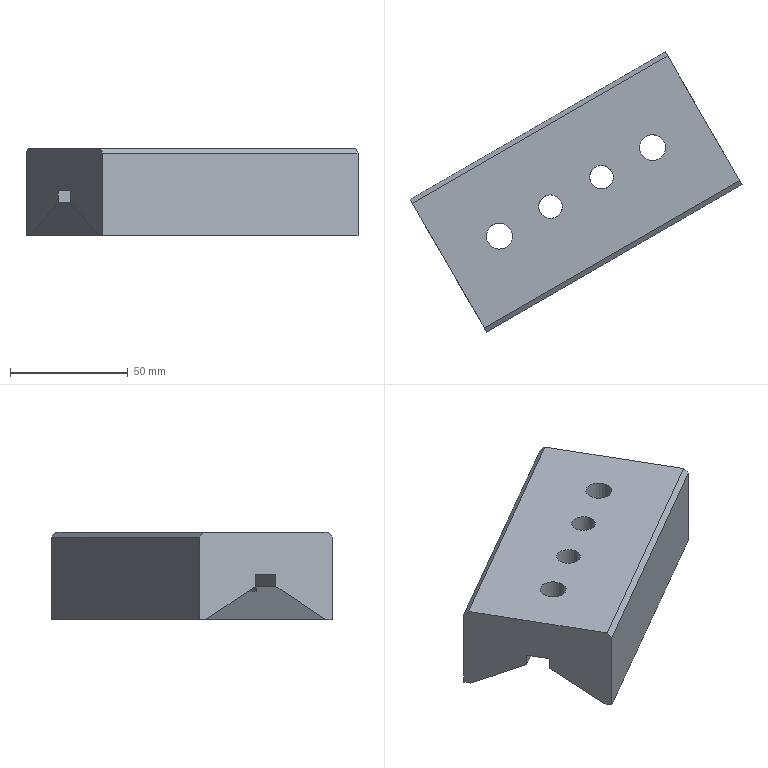Part | NX | features solid 2 | 1 solid | 30 faces | box 140.753 x 118.792 x 37 mm | volume 223802 mm3 | plane 24 | cylinder 6 | commonest cylinder face diameters 10 x2 11 x2 17.5 x2
STEP:
#1=CARTESIAN_POINT('',(-902.48,110.974,-228.));
#2=VERTEX_POINT('',#1);
#3=CARTESIAN_POINT('',(-917.912,102.065,-228.));
#4=VERTEX_POINT('',#3);
#5=CARTESIAN_POINT('',(-902.48,110.974,-228.));
#6=DIRECTION('',(-0.866,-0.5,0.));
#7=VECTOR('',#6,1000.);
#8=LINE('',#5,#7);
#9=EDGE_CURVE('',#2,#4,#8,.T.);
#10=ORIENTED_EDGE('',*,*,#9,.F.);
#11=CARTESIAN_POINT('',(-902.48,110.974,-232.887));
#12=VERTEX_POINT('',#11);
#13=CARTESIAN_POINT('',(-902.48,110.974,-228.));
#14=DIRECTION('',(0.,0.,-1.));
#15=VECTOR('',#14,1000.);
#16=LINE('',#13,#15);
#17=EDGE_CURVE('',#2,#12,#16,.T.);
#18=ORIENTED_EDGE('',*,*,#17,.T.);
#19=CARTESIAN_POINT('',(-917.912,102.065,-232.887));
#20=VERTEX_POINT('',#19);
#21=CARTESIAN_POINT('',(-902.48,110.974,-232.887));
#22=DIRECTION('',(-0.866,-0.5,0.));
#23=VECTOR('',#22,1000.);
#24=LINE('',#21,#23);
#25=EDGE_CURVE('',#12,#20,#24,.T.);
#26=ORIENTED_EDGE('',*,*,#25,.T.);
#27=CARTESIAN_POINT('',(-917.912,102.065,-220.));
#28=DIRECTION('',(0.,0.,-1.));
#29=VECTOR('',#28,1000.);
#30=LINE('',#27,#29);
#31=EDGE_CURVE('',#4,#20,#30,.T.);
#32=ORIENTED_EDGE('',*,*,#31,.F.);
#33=EDGE_LOOP('',(#10,#18,#26,#32));
#34=FACE_BOUND('',#33,.T.);
#35=CARTESIAN_POINT('',(-902.48,110.974,-228.));
#36=DIRECTION('',(0.5,-0.866,0.));
#37=DIRECTION('',(0.,0.,1.));
#38=AXIS2_PLACEMENT_3D('',#35,#36,#37);
#39=PLANE('',#38);
#40=ADVANCED_FACE('',(#34),#39,.F.);
#41=CARTESIAN_POINT('',(-930.349,94.884,-228.));
#42=VERTEX_POINT('',#41);
#43=CARTESIAN_POINT('',(-945.781,85.974,-228.));
#44=VERTEX_POINT('',#43);
#45=CARTESIAN_POINT('',(-902.48,110.974,-228.));
#46=DIRECTION('',(-0.866,-0.5,0.));
#47=VECTOR('',#46,1000.);
#48=LINE('',#45,#47);
#49=EDGE_CURVE('',#42,#44,#48,.T.);
#50=ORIENTED_EDGE('',*,*,#49,.T.);
#51=CARTESIAN_POINT('',(-950.781,94.634,-228.));
#52=VERTEX_POINT('',#51);
#53=CARTESIAN_POINT('',(-948.281,90.304,-228.));
#54=DIRECTION('',(0.,0.,-1.));
#55=DIRECTION('',(0.866,0.5,0.));
#56=AXIS2_PLACEMENT_3D('',#53,#54,#55);
#57=CIRCLE('',#56,5.);
#58=EDGE_CURVE('',#52,#44,#57,.T.);
#59=ORIENTED_EDGE('',*,*,#58,.F.);
#60=CARTESIAN_POINT('',(-935.349,103.544,-228.));
#61=VERTEX_POINT('',#60);
#62=CARTESIAN_POINT('',(-907.48,119.634,-228.));
#63=DIRECTION('',(-0.866,-0.5,0.));
#64=VECTOR('',#63,1000.);
#65=LINE('',#62,#64);
#66=EDGE_CURVE('',#61,#52,#65,.T.);
#67=ORIENTED_EDGE('',*,*,#66,.F.);
#68=CARTESIAN_POINT('',(-926.631,102.804,-228.));
#69=DIRECTION('',(0.,0.,-1.));
#70=DIRECTION('',(0.866,0.5,0.));
#71=AXIS2_PLACEMENT_3D('',#68,#69,#70);
#72=CIRCLE('',#71,8.75);
#73=EDGE_CURVE('',#42,#61,#72,.T.);
#74=ORIENTED_EDGE('',*,*,#73,.F.);
#75=EDGE_LOOP('',(#50,#59,#67,#74));
#76=FACE_BOUND('',#75,.T.);
#77=CARTESIAN_POINT('',(-907.48,119.634,-228.));
#78=DIRECTION('',(0.,0.,1.));
#79=DIRECTION('',(0.866,0.5,0.));
#80=AXIS2_PLACEMENT_3D('',#77,#78,#79);
#81=PLANE('',#80);
#82=ADVANCED_FACE('',(#76),#81,.F.);
#83=ORIENTED_EDGE('',*,*,#66,.T.);
#84=CARTESIAN_POINT('',(-972.432,82.134,-228.));
#85=VERTEX_POINT('',#84);
#86=CARTESIAN_POINT('',(-907.48,119.634,-228.));
#87=DIRECTION('',(-0.866,-0.5,0.));
#88=VECTOR('',#87,1000.);
#89=LINE('',#86,#88);
#90=EDGE_CURVE('',#52,#85,#89,.T.);
#91=ORIENTED_EDGE('',*,*,#90,.T.);
#92=CARTESIAN_POINT('',(-987.864,73.225,-228.));
#93=VERTEX_POINT('',#92);
#94=CARTESIAN_POINT('',(-907.48,119.634,-228.));
#95=DIRECTION('',(-0.866,-0.5,0.));
#96=VECTOR('',#95,1000.);
#97=LINE('',#94,#96);
#98=EDGE_CURVE('',#85,#93,#97,.T.);
#99=ORIENTED_EDGE('',*,*,#98,.T.);
#100=CARTESIAN_POINT('',(-987.864,73.225,-232.887));
#101=VERTEX_POINT('',#100);
#102=CARTESIAN_POINT('',(-987.864,73.225,-220.));
#103=DIRECTION('',(0.,0.,-1.));
#104=VECTOR('',#103,1000.);
#105=LINE('',#102,#104);
#106=EDGE_CURVE('',#101,#93,#105,.F.);
#107=ORIENTED_EDGE('',*,*,#106,.F.);
#108=CARTESIAN_POINT('',(-935.349,103.544,-232.887));
#109=VERTEX_POINT('',#108);
#110=CARTESIAN_POINT('',(-907.48,119.634,-232.887));
#111=DIRECTION('',(-0.866,-0.5,0.));
#112=VECTOR('',#111,1000.);
#113=LINE('',#110,#112);
#114=EDGE_CURVE('',#109,#101,#113,.T.);
#115=ORIENTED_EDGE('',*,*,#114,.F.);
#116=CARTESIAN_POINT('',(-935.349,103.544,-220.));
#117=DIRECTION('',(0.,0.,-1.));
#118=VECTOR('',#117,1000.);
#119=LINE('',#116,#118);
#120=EDGE_CURVE('',#61,#109,#119,.T.);
#121=ORIENTED_EDGE('',*,*,#120,.F.);
#122=EDGE_LOOP('',(#83,#91,#99,#107,#115,#121));
#123=FACE_BOUND('',#122,.T.);
#124=CARTESIAN_POINT('',(-907.48,119.634,-232.887));
#125=DIRECTION('',(-0.5,0.866,0.));
#126=DIRECTION('',(0.,0.,-1.));
#127=AXIS2_PLACEMENT_3D('',#124,#125,#126);
#128=PLANE('',#127);
#129=ADVANCED_FACE('',(#123),#128,.F.);
#130=CARTESIAN_POINT('',(-967.432,73.474,-228.));
#131=VERTEX_POINT('',#130);
#132=CARTESIAN_POINT('',(-902.48,110.974,-228.));
#133=DIRECTION('',(-0.866,-0.5,0.));
#134=VECTOR('',#133,1000.);
#135=LINE('',#132,#134);
#136=EDGE_CURVE('',#44,#131,#135,.T.);
#137=ORIENTED_EDGE('',*,*,#136,.T.);
#138=CARTESIAN_POINT('',(-969.932,77.804,-228.));
#139=DIRECTION('',(0.,0.,-1.));
#140=DIRECTION('',(0.866,0.5,0.));
#141=AXIS2_PLACEMENT_3D('',#138,#139,#140);
#142=CIRCLE('',#141,5.);
#143=EDGE_CURVE('',#85,#131,#142,.T.);
#144=ORIENTED_EDGE('',*,*,#143,.F.);
#145=ORIENTED_EDGE('',*,*,#90,.F.);
#146=CARTESIAN_POINT('',(-948.281,90.304,-228.));
#147=DIRECTION('',(0.,0.,-1.));
#148=DIRECTION('',(0.866,0.5,0.));
#149=AXIS2_PLACEMENT_3D('',#146,#147,#148);
#150=CIRCLE('',#149,5.);
#151=EDGE_CURVE('',#44,#52,#150,.T.);
#152=ORIENTED_EDGE('',*,*,#151,.F.);
#153=EDGE_LOOP('',(#137,#144,#145,#152));
#154=FACE_BOUND('',#153,.T.);
#155=CARTESIAN_POINT('',(-907.48,119.634,-228.));
#156=DIRECTION('',(0.,0.,1.));
#157=DIRECTION('',(0.866,0.5,0.));
#158=AXIS2_PLACEMENT_3D('',#155,#156,#157);
#159=PLANE('',#158);
#160=ADVANCED_FACE('',(#154),#159,.F.);
#161=CARTESIAN_POINT('',(-982.864,64.565,-228.));
#162=VERTEX_POINT('',#161);
#163=CARTESIAN_POINT('',(-902.48,110.974,-228.));
#164=DIRECTION('',(-0.866,-0.5,0.));
#165=VECTOR('',#164,1000.);
#166=LINE('',#163,#165);
#167=EDGE_CURVE('',#131,#162,#166,.T.);
#168=ORIENTED_EDGE('',*,*,#167,.T.);
#169=CARTESIAN_POINT('',(-991.583,65.304,-228.));
#170=DIRECTION('',(0.,0.,-1.));
#171=DIRECTION('',(0.866,0.5,0.));
#172=AXIS2_PLACEMENT_3D('',#169,#170,#171);
#173=CIRCLE('',#172,8.75);
#174=EDGE_CURVE('',#93,#162,#173,.T.);
#175=ORIENTED_EDGE('',*,*,#174,.F.);
#176=ORIENTED_EDGE('',*,*,#98,.F.);
#177=CARTESIAN_POINT('',(-969.932,77.804,-228.));
#178=DIRECTION('',(0.,0.,-1.));
#179=DIRECTION('',(0.866,0.5,0.));
#180=AXIS2_PLACEMENT_3D('',#177,#178,#179);
#181=CIRCLE('',#180,5.);
#182=EDGE_CURVE('',#131,#85,#181,.T.);
#183=ORIENTED_EDGE('',*,*,#182,.F.);
#184=EDGE_LOOP('',(#168,#175,#176,#183));
#185=FACE_BOUND('',#184,.T.);
#186=CARTESIAN_POINT('',(-907.48,119.634,-228.));
#187=DIRECTION('',(0.,0.,1.));
#188=DIRECTION('',(0.866,0.5,0.));
#189=AXIS2_PLACEMENT_3D('',#186,#187,#188);
#190=PLANE('',#189);
#191=ADVANCED_FACE('',(#185),#190,.F.);
#192=CARTESIAN_POINT('',(-930.349,94.884,-232.887));
#193=VERTEX_POINT('',#192);
#194=CARTESIAN_POINT('',(-982.864,64.565,-232.887));
#195=VERTEX_POINT('',#194);
#196=CARTESIAN_POINT('',(-902.48,110.974,-232.887));
#197=DIRECTION('',(-0.866,-0.5,0.));
#198=VECTOR('',#197,1000.);
#199=LINE('',#196,#198);
#200=EDGE_CURVE('',#193,#195,#199,.T.);
#201=ORIENTED_EDGE('',*,*,#200,.T.);
#202=CARTESIAN_POINT('',(-982.864,64.565,-220.));
#203=DIRECTION('',(0.,0.,-1.));
#204=VECTOR('',#203,1000.);
#205=LINE('',#202,#204);
#206=EDGE_CURVE('',#162,#195,#205,.T.);
#207=ORIENTED_EDGE('',*,*,#206,.F.);
#208=ORIENTED_EDGE('',*,*,#167,.F.);
#209=ORIENTED_EDGE('',*,*,#136,.F.);
#210=ORIENTED_EDGE('',*,*,#49,.F.);
#211=CARTESIAN_POINT('',(-930.349,94.884,-220.));
#212=DIRECTION('',(0.,0.,-1.));
#213=VECTOR('',#212,1000.);
#214=LINE('',#211,#213);
#215=EDGE_CURVE('',#193,#42,#214,.F.);
#216=ORIENTED_EDGE('',*,*,#215,.F.);
#217=EDGE_LOOP('',(#201,#207,#208,#209,#210,#216));
#218=FACE_BOUND('',#217,.T.);
#219=CARTESIAN_POINT('',(-902.48,110.974,-228.));
#220=DIRECTION('',(0.5,-0.866,0.));
#221=DIRECTION('',(0.,0.,1.));
#222=AXIS2_PLACEMENT_3D('',#219,#220,#221);
#223=PLANE('',#222);
#224=ADVANCED_FACE('',(#218),#223,.F.);
#225=CARTESIAN_POINT('',(-995.301,57.384,-228.));
#226=VERTEX_POINT('',#225);
#227=CARTESIAN_POINT('',(-1010.733,48.474,-228.));
#228=VERTEX_POINT('',#227);
#229=CARTESIAN_POINT('',(-902.48,110.974,-228.));
#230=DIRECTION('',(-0.866,-0.5,0.));
#231=VECTOR('',#230,1000.);
#232=LINE('',#229,#231);
#233=EDGE_CURVE('',#226,#228,#232,.T.);
#234=ORIENTED_EDGE('',*,*,#233,.T.);
#235=CARTESIAN_POINT('',(-1015.733,57.134,-228.));
#236=VERTEX_POINT('',#235);
#237=CARTESIAN_POINT('',(-1015.733,57.134,-228.));
#238=DIRECTION('',(0.5,-0.866,0.));
#239=VECTOR('',#238,1000.);
#240=LINE('',#237,#239);
#241=EDGE_CURVE('',#236,#228,#240,.T.);
#242=ORIENTED_EDGE('',*,*,#241,.F.);
#243=CARTESIAN_POINT('',(-1000.301,66.044,-228.));
#244=VERTEX_POINT('',#243);
#245=CARTESIAN_POINT('',(-907.48,119.634,-228.));
#246=DIRECTION('',(-0.866,-0.5,0.));
#247=VECTOR('',#246,1000.);
#248=LINE('',#245,#247);
#249=EDGE_CURVE('',#244,#236,#248,.T.);
#250=ORIENTED_EDGE('',*,*,#249,.F.);
#251=CARTESIAN_POINT('',(-991.583,65.304,-228.));
#252=DIRECTION('',(0.,0.,-1.));
#253=DIRECTION('',(0.866,0.5,0.));
#254=AXIS2_PLACEMENT_3D('',#251,#252,#253);
#255=CIRCLE('',#254,8.75);
#256=EDGE_CURVE('',#226,#244,#255,.T.);
#257=ORIENTED_EDGE('',*,*,#256,.F.);
#258=EDGE_LOOP('',(#234,#242,#250,#257));
#259=FACE_BOUND('',#258,.T.);
#260=CARTESIAN_POINT('',(-907.48,119.634,-228.));
#261=DIRECTION('',(0.,0.,1.));
#262=DIRECTION('',(0.866,0.5,0.));
#263=AXIS2_PLACEMENT_3D('',#260,#261,#262);
#264=PLANE('',#263);
#265=ADVANCED_FACE('',(#259),#264,.F.);
#266=ORIENTED_EDGE('',*,*,#249,.T.);
#267=CARTESIAN_POINT('',(-1015.733,57.134,-232.887));
#268=VERTEX_POINT('',#267);
#269=CARTESIAN_POINT('',(-1015.733,57.134,-232.887));
#270=DIRECTION('',(0.,0.,1.));
#271=VECTOR('',#270,1000.);
#272=LINE('',#269,#271);
#273=EDGE_CURVE('',#268,#236,#272,.T.);
#274=ORIENTED_EDGE('',*,*,#273,.F.);
#275=CARTESIAN_POINT('',(-1000.301,66.044,-232.887));
#276=VERTEX_POINT('',#275);
#277=CARTESIAN_POINT('',(-907.48,119.634,-232.887));
#278=DIRECTION('',(-0.866,-0.5,0.));
#279=VECTOR('',#278,1000.);
#280=LINE('',#277,#279);
#281=EDGE_CURVE('',#276,#268,#280,.T.);
#282=ORIENTED_EDGE('',*,*,#281,.F.);
#283=CARTESIAN_POINT('',(-1000.301,66.044,-220.));
#284=DIRECTION('',(0.,0.,-1.));
#285=VECTOR('',#284,1000.);
#286=LINE('',#283,#285);
#287=EDGE_CURVE('',#244,#276,#286,.T.);
#288=ORIENTED_EDGE('',*,*,#287,.F.);
#289=EDGE_LOOP('',(#266,#274,#282,#288));
#290=FACE_BOUND('',#289,.T.);
#291=CARTESIAN_POINT('',(-907.48,119.634,-232.887));
#292=DIRECTION('',(-0.5,0.866,0.));
#293=DIRECTION('',(0.,0.,-1.));
#294=AXIS2_PLACEMENT_3D('',#291,#292,#293);
#295=PLANE('',#294);
#296=ADVANCED_FACE('',(#290),#295,.F.);
#297=CARTESIAN_POINT('',(-931.394,100.054,-210.));
#298=VERTEX_POINT('',#297);
#299=CARTESIAN_POINT('',(-926.631,102.804,-210.));
#300=DIRECTION('',(0.,0.,1.));
#301=DIRECTION('',(-0.866,-0.5,0.));
#302=AXIS2_PLACEMENT_3D('',#299,#300,#301);
#303=CIRCLE('',#302,5.5);
#304=EDGE_CURVE('',#298,#298,#303,.T.);
#305=ORIENTED_EDGE('',*,*,#304,.F.);
#306=EDGE_LOOP('',(#305));
#307=FACE_BOUND('',#306,.T.);
#308=CARTESIAN_POINT('',(-952.612,87.804,-210.));
#309=VERTEX_POINT('',#308);
#310=CARTESIAN_POINT('',(-948.281,90.304,-210.));
#311=DIRECTION('',(0.,0.,1.));
#312=DIRECTION('',(-0.866,-0.5,0.));
#313=AXIS2_PLACEMENT_3D('',#310,#311,#312);
#314=CIRCLE('',#313,5.);
#315=EDGE_CURVE('',#309,#309,#314,.T.);
#316=ORIENTED_EDGE('',*,*,#315,.F.);
#317=EDGE_LOOP('',(#316));
#318=FACE_BOUND('',#317,.T.);
#319=CARTESIAN_POINT('',(-974.262,75.304,-210.));
#320=VERTEX_POINT('',#319);
#321=CARTESIAN_POINT('',(-969.932,77.804,-210.));
#322=DIRECTION('',(0.,0.,1.));
#323=DIRECTION('',(-0.866,-0.5,0.));
#324=AXIS2_PLACEMENT_3D('',#321,#322,#323);
#325=CIRCLE('',#324,5.);
#326=EDGE_CURVE('',#320,#320,#325,.T.);
#327=ORIENTED_EDGE('',*,*,#326,.F.);
#328=EDGE_LOOP('',(#327));
#329=FACE_BOUND('',#328,.T.);
#330=CARTESIAN_POINT('',(-996.346,62.554,-210.));
#331=VERTEX_POINT('',#330);
#332=CARTESIAN_POINT('',(-991.583,65.304,-210.));
#333=DIRECTION('',(0.,0.,1.));
#334=DIRECTION('',(-0.866,-0.5,0.));
#335=AXIS2_PLACEMENT_3D('',#332,#333,#334);
#336=CIRCLE('',#335,5.5);
#337=EDGE_CURVE('',#331,#331,#336,.T.);
#338=ORIENTED_EDGE('',*,*,#337,.F.);
#339=EDGE_LOOP('',(#338));
#340=FACE_BOUND('',#339,.T.);
#341=CARTESIAN_POINT('',(-920.23,141.718,-210.));
#342=VERTEX_POINT('',#341);
#343=CARTESIAN_POINT('',(-889.73,88.891,-210.));
#344=VERTEX_POINT('',#343);
#345=CARTESIAN_POINT('',(-921.23,143.45,-210.));
#346=DIRECTION('',(0.5,-0.866,0.));
#347=VECTOR('',#346,1000.);
#348=LINE('',#345,#347);
#349=EDGE_CURVE('',#342,#344,#348,.T.);
#350=ORIENTED_EDGE('',*,*,#349,.F.);
#351=CARTESIAN_POINT('',(-1028.483,79.218,-210.));
#352=VERTEX_POINT('',#351);
#353=CARTESIAN_POINT('',(-920.23,141.718,-210.));
#354=DIRECTION('',(0.866,0.5,0.));
#355=VECTOR('',#354,1000.);
#356=LINE('',#353,#355);
#357=EDGE_CURVE('',#352,#342,#356,.T.);
#358=ORIENTED_EDGE('',*,*,#357,.F.);
#359=CARTESIAN_POINT('',(-997.983,26.391,-210.));
#360=VERTEX_POINT('',#359);
#361=CARTESIAN_POINT('',(-1029.483,80.95,-210.));
#362=DIRECTION('',(0.5,-0.866,0.));
#363=VECTOR('',#362,1000.);
#364=LINE('',#361,#363);
#365=EDGE_CURVE('',#352,#360,#364,.T.);
#366=ORIENTED_EDGE('',*,*,#365,.T.);
#367=CARTESIAN_POINT('',(-889.73,88.891,-210.));
#368=DIRECTION('',(-0.866,-0.5,0.));
#369=VECTOR('',#368,1000.);
#370=LINE('',#367,#369);
#371=EDGE_CURVE('',#344,#360,#370,.T.);
#372=ORIENTED_EDGE('',*,*,#371,.F.);
#373=EDGE_LOOP('',(#350,#358,#366,#372));
#374=FACE_BOUND('',#373,.T.);
#375=CARTESIAN_POINT('',(-921.23,143.45,-210.));
#376=DIRECTION('',(0.,0.,1.));
#377=DIRECTION('',(-0.5,0.866,0.));
#378=AXIS2_PLACEMENT_3D('',#375,#376,#377);
#379=PLANE('',#378);
#380=ADVANCED_FACE('',(#307,#318,#329,#340,#374),#379,.T.);
#381=CARTESIAN_POINT('',(-996.983,24.658,-212.));
#382=VERTEX_POINT('',#381);
#383=CARTESIAN_POINT('',(-996.983,24.658,-247.));
#384=VERTEX_POINT('',#383);
#385=CARTESIAN_POINT('',(-996.983,24.658,-210.));
#386=DIRECTION('',(0.,0.,-1.));
#387=VECTOR('',#386,1000.);
#388=LINE('',#385,#387);
#389=EDGE_CURVE('',#382,#384,#388,.T.);
#390=ORIENTED_EDGE('',*,*,#389,.T.);
#391=CARTESIAN_POINT('',(-888.73,87.158,-247.));
#392=VERTEX_POINT('',#391);
#393=CARTESIAN_POINT('',(-888.73,87.158,-247.));
#394=DIRECTION('',(-0.866,-0.5,0.));
#395=VECTOR('',#394,1000.);
#396=LINE('',#393,#395);
#397=EDGE_CURVE('',#392,#384,#396,.T.);
#398=ORIENTED_EDGE('',*,*,#397,.F.);
#399=CARTESIAN_POINT('',(-888.73,87.158,-212.));
#400=VERTEX_POINT('',#399);
#401=CARTESIAN_POINT('',(-888.73,87.158,-210.));
#402=DIRECTION('',(0.,0.,-1.));
#403=VECTOR('',#402,1000.);
#404=LINE('',#401,#403);
#405=EDGE_CURVE('',#400,#392,#404,.T.);
#406=ORIENTED_EDGE('',*,*,#405,.F.);
#407=CARTESIAN_POINT('',(-888.73,87.158,-212.));
#408=DIRECTION('',(0.866,0.5,0.));
#409=VECTOR('',#408,1000.);
#410=LINE('',#407,#409);
#411=EDGE_CURVE('',#382,#400,#410,.T.);
#412=ORIENTED_EDGE('',*,*,#411,.F.);
#413=EDGE_LOOP('',(#390,#398,#406,#412));
#414=FACE_BOUND('',#413,.T.);
#415=CARTESIAN_POINT('',(-888.73,87.158,-210.));
#416=DIRECTION('',(0.5,-0.866,0.));
#417=DIRECTION('',(0.,0.,1.));
#418=AXIS2_PLACEMENT_3D('',#415,#416,#417);
#419=PLANE('',#418);
#420=ADVANCED_FACE('',(#414),#419,.T.);
#421=CARTESIAN_POINT('',(-998.511,27.304,-247.));
#422=VERTEX_POINT('',#421);
#423=CARTESIAN_POINT('',(-996.983,24.658,-247.));
#424=DIRECTION('',(-0.5,0.866,0.));
#425=VECTOR('',#424,1000.);
#426=LINE('',#423,#425);
#427=EDGE_CURVE('',#384,#422,#426,.T.);
#428=ORIENTED_EDGE('',*,*,#427,.T.);
#429=CARTESIAN_POINT('',(-890.258,89.804,-247.));
#430=VERTEX_POINT('',#429);
#431=CARTESIAN_POINT('',(-890.258,89.804,-247.));
#432=DIRECTION('',(-0.866,-0.5,0.));
#433=VECTOR('',#432,1000.);
#434=LINE('',#431,#433);
#435=EDGE_CURVE('',#430,#422,#434,.T.);
#436=ORIENTED_EDGE('',*,*,#435,.F.);
#437=CARTESIAN_POINT('',(-888.73,87.158,-247.));
#438=DIRECTION('',(-0.5,0.866,0.));
#439=VECTOR('',#438,1000.);
#440=LINE('',#437,#439);
#441=EDGE_CURVE('',#392,#430,#440,.T.);
#442=ORIENTED_EDGE('',*,*,#441,.F.);
#443=ORIENTED_EDGE('',*,*,#397,.T.);
#444=EDGE_LOOP('',(#428,#436,#442,#443));
#445=FACE_BOUND('',#444,.T.);
#446=CARTESIAN_POINT('',(-888.73,87.158,-247.));
#447=DIRECTION('',(0.,0.,-1.));
#448=DIRECTION('',(0.5,-0.866,0.));
#449=AXIS2_PLACEMENT_3D('',#446,#447,#448);
#450=PLANE('',#449);
#451=ADVANCED_FACE('',(#445),#450,.T.);
#452=ORIENTED_EDGE('',*,*,#25,.F.);
#453=CARTESIAN_POINT('',(-902.48,110.974,-232.887));
#454=DIRECTION('',(0.433,-0.75,-0.5));
#455=VECTOR('',#454,1000.);
#456=LINE('',#453,#455);
#457=EDGE_CURVE('',#12,#430,#456,.T.);
#458=ORIENTED_EDGE('',*,*,#457,.T.);
#459=ORIENTED_EDGE('',*,*,#435,.T.);
#460=CARTESIAN_POINT('',(-1010.733,48.474,-232.887));
#461=VERTEX_POINT('',#460);
#462=CARTESIAN_POINT('',(-1010.733,48.474,-232.887));
#463=DIRECTION('',(0.433,-0.75,-0.5));
#464=VECTOR('',#463,1000.);
#465=LINE('',#462,#464);
#466=EDGE_CURVE('',#461,#422,#465,.T.);
#467=ORIENTED_EDGE('',*,*,#466,.F.);
#468=CARTESIAN_POINT('',(-995.301,57.384,-232.887));
#469=VERTEX_POINT('',#468);
#470=CARTESIAN_POINT('',(-902.48,110.974,-232.887));
#471=DIRECTION('',(-0.866,-0.5,0.));
#472=VECTOR('',#471,1000.);
#473=LINE('',#470,#472);
#474=EDGE_CURVE('',#469,#461,#473,.T.);
#475=ORIENTED_EDGE('',*,*,#474,.F.);
#476=CARTESIAN_POINT('',(-991.583,65.304,-230.));
#477=DIRECTION('',(-0.25,0.433,-0.866));
#478=DIRECTION('',(0.433,-0.75,-0.5));
#479=AXIS2_PLACEMENT_3D('',#476,#477,#478);
#480=ELLIPSE('',#479,10.104,8.75);
#481=EDGE_CURVE('',#195,#469,#480,.T.);
#482=ORIENTED_EDGE('',*,*,#481,.F.);
#483=ORIENTED_EDGE('',*,*,#200,.F.);
#484=CARTESIAN_POINT('',(-926.631,102.804,-230.));
#485=DIRECTION('',(-0.25,0.433,-0.866));
#486=DIRECTION('',(0.433,-0.75,-0.5));
#487=AXIS2_PLACEMENT_3D('',#484,#485,#486);
#488=ELLIPSE('',#487,10.104,8.75);
#489=EDGE_CURVE('',#20,#193,#488,.T.);
#490=ORIENTED_EDGE('',*,*,#489,.F.);
#491=EDGE_LOOP('',(#452,#458,#459,#467,#475,#482,#483,#490));
#492=FACE_BOUND('',#491,.T.);
#493=CARTESIAN_POINT('',(-902.48,110.974,-232.887));
#494=DIRECTION('',(0.25,-0.433,0.866));
#495=DIRECTION('',(-0.433,0.75,0.5));
#496=AXIS2_PLACEMENT_3D('',#493,#494,#495);
#497=PLANE('',#496);
#498=ADVANCED_FACE('',(#492),#497,.F.);
#499=ORIENTED_EDGE('',*,*,#474,.T.);
#500=CARTESIAN_POINT('',(-1010.733,48.474,-228.));
#501=DIRECTION('',(0.,0.,-1.));
#502=VECTOR('',#501,1000.);
#503=LINE('',#500,#502);
#504=EDGE_CURVE('',#228,#461,#503,.T.);
#505=ORIENTED_EDGE('',*,*,#504,.F.);
#506=ORIENTED_EDGE('',*,*,#233,.F.);
#507=CARTESIAN_POINT('',(-995.301,57.384,-220.));
#508=DIRECTION('',(0.,0.,-1.));
#509=VECTOR('',#508,1000.);
#510=LINE('',#507,#509);
#511=EDGE_CURVE('',#469,#226,#510,.F.);
#512=ORIENTED_EDGE('',*,*,#511,.F.);
#513=EDGE_LOOP('',(#499,#505,#506,#512));
#514=FACE_BOUND('',#513,.T.);
#515=CARTESIAN_POINT('',(-902.48,110.974,-228.));
#516=DIRECTION('',(0.5,-0.866,0.));
#517=DIRECTION('',(0.,0.,1.));
#518=AXIS2_PLACEMENT_3D('',#515,#516,#517);
#519=PLANE('',#518);
#520=ADVANCED_FACE('',(#514),#519,.F.);
#521=CARTESIAN_POINT('',(-907.48,119.634,-228.));
#522=VERTEX_POINT('',#521);
#523=CARTESIAN_POINT('',(-922.912,110.725,-228.));
#524=VERTEX_POINT('',#523);
#525=CARTESIAN_POINT('',(-907.48,119.634,-228.));
#526=DIRECTION('',(-0.866,-0.5,0.));
#527=VECTOR('',#526,1000.);
#528=LINE('',#525,#527);
#529=EDGE_CURVE('',#522,#524,#528,.T.);
#530=ORIENTED_EDGE('',*,*,#529,.F.);
#531=CARTESIAN_POINT('',(-907.48,119.634,-228.));
#532=DIRECTION('',(0.5,-0.866,0.));
#533=VECTOR('',#532,1000.);
#534=LINE('',#531,#533);
#535=EDGE_CURVE('',#522,#2,#534,.T.);
#536=ORIENTED_EDGE('',*,*,#535,.T.);
#537=ORIENTED_EDGE('',*,*,#9,.T.);
#538=CARTESIAN_POINT('',(-926.631,102.804,-228.));
#539=DIRECTION('',(0.,0.,-1.));
#540=DIRECTION('',(0.866,0.5,0.));
#541=AXIS2_PLACEMENT_3D('',#538,#539,#540);
#542=CIRCLE('',#541,8.75);
#543=EDGE_CURVE('',#524,#4,#542,.T.);
#544=ORIENTED_EDGE('',*,*,#543,.F.);
#545=EDGE_LOOP('',(#530,#536,#537,#544));
#546=FACE_BOUND('',#545,.T.);
#547=CARTESIAN_POINT('',(-907.48,119.634,-228.));
#548=DIRECTION('',(0.,0.,1.));
#549=DIRECTION('',(0.866,0.5,0.));
#550=AXIS2_PLACEMENT_3D('',#547,#548,#549);
#551=PLANE('',#550);
#552=ADVANCED_FACE('',(#546),#551,.F.);
#553=CARTESIAN_POINT('',(-907.48,119.634,-232.887));
#554=VERTEX_POINT('',#553);
#555=CARTESIAN_POINT('',(-922.912,110.725,-232.887));
#556=VERTEX_POINT('',#555);
#557=CARTESIAN_POINT('',(-907.48,119.634,-232.887));
#558=DIRECTION('',(-0.866,-0.5,0.));
#559=VECTOR('',#558,1000.);
#560=LINE('',#557,#559);
#561=EDGE_CURVE('',#554,#556,#560,.T.);
#562=ORIENTED_EDGE('',*,*,#561,.F.);
#563=CARTESIAN_POINT('',(-907.48,119.634,-232.887));
#564=DIRECTION('',(0.,0.,1.));
#565=VECTOR('',#564,1000.);
#566=LINE('',#563,#565);
#567=EDGE_CURVE('',#554,#522,#566,.T.);
#568=ORIENTED_EDGE('',*,*,#567,.T.);
#569=ORIENTED_EDGE('',*,*,#529,.T.);
#570=CARTESIAN_POINT('',(-922.912,110.725,-220.));
#571=DIRECTION('',(0.,0.,-1.));
#572=VECTOR('',#571,1000.);
#573=LINE('',#570,#572);
#574=EDGE_CURVE('',#556,#524,#573,.F.);
#575=ORIENTED_EDGE('',*,*,#574,.F.);
#576=EDGE_LOOP('',(#562,#568,#569,#575));
#577=FACE_BOUND('',#576,.T.);
#578=CARTESIAN_POINT('',(-907.48,119.634,-232.887));
#579=DIRECTION('',(-0.5,0.866,0.));
#580=DIRECTION('',(0.,0.,-1.));
#581=AXIS2_PLACEMENT_3D('',#578,#579,#580);
#582=PLANE('',#581);
#583=ADVANCED_FACE('',(#577),#582,.F.);
#584=ORIENTED_EDGE('',*,*,#114,.T.);
#585=CARTESIAN_POINT('',(-991.583,65.304,-230.));
#586=DIRECTION('',(0.25,-0.433,-0.866));
#587=DIRECTION('',(-0.433,0.75,-0.5));
#588=AXIS2_PLACEMENT_3D('',#585,#586,#587);
#589=ELLIPSE('',#588,10.104,8.75);
#590=EDGE_CURVE('',#276,#101,#589,.T.);
#591=ORIENTED_EDGE('',*,*,#590,.F.);
#592=ORIENTED_EDGE('',*,*,#281,.T.);
#593=CARTESIAN_POINT('',(-1027.956,78.304,-247.));
#594=VERTEX_POINT('',#593);
#595=CARTESIAN_POINT('',(-1027.956,78.304,-247.));
#596=DIRECTION('',(0.433,-0.75,0.5));
#597=VECTOR('',#596,1000.);
#598=LINE('',#595,#597);
#599=EDGE_CURVE('',#594,#268,#598,.T.);
#600=ORIENTED_EDGE('',*,*,#599,.F.);
#601=CARTESIAN_POINT('',(-919.703,140.804,-247.));
#602=VERTEX_POINT('',#601);
#603=CARTESIAN_POINT('',(-919.703,140.804,-247.));
#604=DIRECTION('',(-0.866,-0.5,0.));
#605=VECTOR('',#604,1000.);
#606=LINE('',#603,#605);
#607=EDGE_CURVE('',#602,#594,#606,.T.);
#608=ORIENTED_EDGE('',*,*,#607,.F.);
#609=CARTESIAN_POINT('',(-919.703,140.804,-247.));
#610=DIRECTION('',(0.433,-0.75,0.5));
#611=VECTOR('',#610,1000.);
#612=LINE('',#609,#611);
#613=EDGE_CURVE('',#602,#554,#612,.T.);
#614=ORIENTED_EDGE('',*,*,#613,.T.);
#615=ORIENTED_EDGE('',*,*,#561,.T.);
#616=CARTESIAN_POINT('',(-926.631,102.804,-230.));
#617=DIRECTION('',(0.25,-0.433,-0.866));
#618=DIRECTION('',(-0.433,0.75,-0.5));
#619=AXIS2_PLACEMENT_3D('',#616,#617,#618);
#620=ELLIPSE('',#619,10.104,8.75);
#621=EDGE_CURVE('',#109,#556,#620,.T.);
#622=ORIENTED_EDGE('',*,*,#621,.F.);
#623=EDGE_LOOP('',(#584,#591,#592,#600,#608,#614,#615,#622));
#624=FACE_BOUND('',#623,.T.);
#625=CARTESIAN_POINT('',(-919.703,140.804,-247.));
#626=DIRECTION('',(-0.25,0.433,0.866));
#627=DIRECTION('',(-0.433,0.75,-0.5));
#628=AXIS2_PLACEMENT_3D('',#625,#626,#627);
#629=PLANE('',#628);
#630=ADVANCED_FACE('',(#624),#629,.F.);
#631=CARTESIAN_POINT('',(-1029.483,80.95,-247.));
#632=VERTEX_POINT('',#631);
#633=CARTESIAN_POINT('',(-1027.956,78.304,-247.));
#634=DIRECTION('',(-0.5,0.866,0.));
#635=VECTOR('',#634,1000.);
#636=LINE('',#633,#635);
#637=EDGE_CURVE('',#594,#632,#636,.T.);
#638=ORIENTED_EDGE('',*,*,#637,.T.);
#639=CARTESIAN_POINT('',(-921.23,143.45,-247.));
#640=VERTEX_POINT('',#639);
#641=CARTESIAN_POINT('',(-921.23,143.45,-247.));
#642=DIRECTION('',(-0.866,-0.5,0.));
#643=VECTOR('',#642,1000.);
#644=LINE('',#641,#643);
#645=EDGE_CURVE('',#640,#632,#644,.T.);
#646=ORIENTED_EDGE('',*,*,#645,.F.);
#647=CARTESIAN_POINT('',(-919.703,140.804,-247.));
#648=DIRECTION('',(-0.5,0.866,0.));
#649=VECTOR('',#648,1000.);
#650=LINE('',#647,#649);
#651=EDGE_CURVE('',#602,#640,#650,.T.);
#652=ORIENTED_EDGE('',*,*,#651,.F.);
#653=ORIENTED_EDGE('',*,*,#607,.T.);
#654=EDGE_LOOP('',(#638,#646,#652,#653));
#655=FACE_BOUND('',#654,.T.);
#656=CARTESIAN_POINT('',(-919.703,140.804,-247.));
#657=DIRECTION('',(0.,0.,-1.));
#658=DIRECTION('',(0.5,-0.866,0.));
#659=AXIS2_PLACEMENT_3D('',#656,#657,#658);
#660=PLANE('',#659);
#661=ADVANCED_FACE('',(#655),#660,.T.);
#662=CARTESIAN_POINT('',(-921.23,143.45,-212.));
#663=VERTEX_POINT('',#662);
#664=CARTESIAN_POINT('',(-921.23,143.45,-247.));
#665=DIRECTION('',(0.,0.,1.));
#666=VECTOR('',#665,1000.);
#667=LINE('',#664,#666);
#668=EDGE_CURVE('',#640,#663,#667,.T.);
#669=ORIENTED_EDGE('',*,*,#668,.F.);
#670=ORIENTED_EDGE('',*,*,#645,.T.);
#671=CARTESIAN_POINT('',(-1029.483,80.95,-212.));
#672=VERTEX_POINT('',#671);
#673=CARTESIAN_POINT('',(-1029.483,80.95,-247.));
#674=DIRECTION('',(0.,0.,1.));
#675=VECTOR('',#674,1000.);
#676=LINE('',#673,#675);
#677=EDGE_CURVE('',#632,#672,#676,.T.);
#678=ORIENTED_EDGE('',*,*,#677,.T.);
#679=CARTESIAN_POINT('',(-921.23,143.45,-212.));
#680=DIRECTION('',(-0.866,-0.5,0.));
#681=VECTOR('',#680,1000.);
#682=LINE('',#679,#681);
#683=EDGE_CURVE('',#663,#672,#682,.T.);
#684=ORIENTED_EDGE('',*,*,#683,.F.);
#685=EDGE_LOOP('',(#669,#670,#678,#684));
#686=FACE_BOUND('',#685,.T.);
#687=CARTESIAN_POINT('',(-921.23,143.45,-247.));
#688=DIRECTION('',(-0.5,0.866,0.));
#689=DIRECTION('',(0.,0.,-1.));
#690=AXIS2_PLACEMENT_3D('',#687,#688,#689);
#691=PLANE('',#690);
#692=ADVANCED_FACE('',(#686),#691,.T.);
#693=ORIENTED_EDGE('',*,*,#405,.T.);
#694=ORIENTED_EDGE('',*,*,#441,.T.);
#695=ORIENTED_EDGE('',*,*,#457,.F.);
#696=ORIENTED_EDGE('',*,*,#17,.F.);
#697=ORIENTED_EDGE('',*,*,#535,.F.);
#698=ORIENTED_EDGE('',*,*,#567,.F.);
#699=ORIENTED_EDGE('',*,*,#613,.F.);
#700=ORIENTED_EDGE('',*,*,#651,.T.);
#701=ORIENTED_EDGE('',*,*,#668,.T.);
#702=CARTESIAN_POINT('',(-921.23,143.45,-212.));
#703=DIRECTION('',(0.3536,-0.6124,0.7071));
#704=VECTOR('',#703,1000.);
#705=LINE('',#702,#704);
#706=EDGE_CURVE('',#342,#663,#705,.F.);
#707=ORIENTED_EDGE('',*,*,#706,.F.);
#708=ORIENTED_EDGE('',*,*,#349,.T.);
#709=CARTESIAN_POINT('',(-889.73,88.891,-210.));
#710=DIRECTION('',(0.3536,-0.6124,-0.7071));
#711=VECTOR('',#710,1000.);
#712=LINE('',#709,#711);
#713=EDGE_CURVE('',#400,#344,#712,.F.);
#714=ORIENTED_EDGE('',*,*,#713,.F.);
#715=EDGE_LOOP('',(#693,#694,#695,#696,#697,#698,#699,#700,#701,#707,#708,#714));
#716=FACE_BOUND('',#715,.T.);
#717=CARTESIAN_POINT('',(-902.48,110.974,-210.));
#718=DIRECTION('',(-0.866,-0.5,0.));
#719=DIRECTION('',(0.,0.,1.));
#720=AXIS2_PLACEMENT_3D('',#717,#718,#719);
#721=PLANE('',#720);
#722=ADVANCED_FACE('',(#716),#721,.F.);
#723=ORIENTED_EDGE('',*,*,#365,.F.);
#724=CARTESIAN_POINT('',(-1019.608,63.846,-192.25));
#725=DIRECTION('',(-0.3536,0.6124,-0.7071));
#726=VECTOR('',#725,1000.);
#727=LINE('',#724,#726);
#728=EDGE_CURVE('',#672,#352,#727,.F.);
#729=ORIENTED_EDGE('',*,*,#728,.F.);
#730=ORIENTED_EDGE('',*,*,#677,.F.);
#731=ORIENTED_EDGE('',*,*,#637,.F.);
#732=ORIENTED_EDGE('',*,*,#599,.T.);
#733=ORIENTED_EDGE('',*,*,#273,.T.);
#734=ORIENTED_EDGE('',*,*,#241,.T.);
#735=ORIENTED_EDGE('',*,*,#504,.T.);
#736=ORIENTED_EDGE('',*,*,#466,.T.);
#737=ORIENTED_EDGE('',*,*,#427,.F.);
#738=ORIENTED_EDGE('',*,*,#389,.F.);
#739=CARTESIAN_POINT('',(-1004.358,37.432,-197.25));
#740=DIRECTION('',(-0.3536,0.6124,0.7071));
#741=VECTOR('',#740,1000.);
#742=LINE('',#739,#741);
#743=EDGE_CURVE('',#360,#382,#742,.F.);
#744=ORIENTED_EDGE('',*,*,#743,.F.);
#745=EDGE_LOOP('',(#723,#729,#730,#731,#732,#733,#734,#735,#736,#737,#738,#744));
#746=FACE_BOUND('',#745,.T.);
#747=CARTESIAN_POINT('',(-1010.733,48.474,-210.));
#748=DIRECTION('',(-0.866,-0.5,0.));
#749=DIRECTION('',(0.,0.,1.));
#750=AXIS2_PLACEMENT_3D('',#747,#748,#749);
#751=PLANE('',#750);
#752=ADVANCED_FACE('',(#746),#751,.T.);
#753=CARTESIAN_POINT('',(-986.82,68.054,-220.));
#754=VERTEX_POINT('',#753);
#755=CARTESIAN_POINT('',(-991.583,65.304,-220.));
#756=DIRECTION('',(0.,0.,-1.));
#757=DIRECTION('',(0.866,0.5,0.));
#758=AXIS2_PLACEMENT_3D('',#755,#756,#757);
#759=CIRCLE('',#758,5.5);
#760=EDGE_CURVE('',#754,#754,#759,.F.);
#761=ORIENTED_EDGE('',*,*,#760,.F.);
#762=EDGE_LOOP('',(#761));
#763=FACE_BOUND('',#762,.T.);
#764=ORIENTED_EDGE('',*,*,#337,.T.);
#765=EDGE_LOOP('',(#764));
#766=FACE_BOUND('',#765,.T.);
#767=CARTESIAN_POINT('',(-991.583,65.304,-210.));
#768=DIRECTION('',(0.,0.,-1.));
#769=DIRECTION('',(-0.866,-0.5,0.));
#770=AXIS2_PLACEMENT_3D('',#767,#768,#769);
#771=CYLINDRICAL_SURFACE('',#770,5.5);
#772=ADVANCED_FACE('',(#763,#766),#771,.F.);
#773=CARTESIAN_POINT('',(-999.16,60.929,-220.));
#774=VERTEX_POINT('',#773);
#775=CARTESIAN_POINT('',(-991.583,65.304,-220.));
#776=DIRECTION('',(0.,0.,1.));
#777=DIRECTION('',(-0.866,-0.5,0.));
#778=AXIS2_PLACEMENT_3D('',#775,#776,#777);
#779=CIRCLE('',#778,8.75);
#780=EDGE_CURVE('',#774,#774,#779,.T.);
#781=ORIENTED_EDGE('',*,*,#780,.T.);
#782=EDGE_LOOP('',(#781));
#783=FACE_BOUND('',#782,.T.);
#784=ORIENTED_EDGE('',*,*,#206,.T.);
#785=ORIENTED_EDGE('',*,*,#481,.T.);
#786=ORIENTED_EDGE('',*,*,#511,.T.);
#787=ORIENTED_EDGE('',*,*,#256,.T.);
#788=ORIENTED_EDGE('',*,*,#287,.T.);
#789=ORIENTED_EDGE('',*,*,#590,.T.);
#790=ORIENTED_EDGE('',*,*,#106,.T.);
#791=ORIENTED_EDGE('',*,*,#174,.T.);
#792=EDGE_LOOP('',(#784,#785,#786,#787,#788,#789,#790,#791));
#793=FACE_BOUND('',#792,.T.);
#794=CARTESIAN_POINT('',(-991.583,65.304,-220.));
#795=DIRECTION('',(0.,0.,-1.));
#796=DIRECTION('',(-0.866,-0.5,0.));
#797=AXIS2_PLACEMENT_3D('',#794,#795,#796);
#798=CYLINDRICAL_SURFACE('',#797,8.75);
#799=ADVANCED_FACE('',(#783,#793),#798,.F.);
#800=ORIENTED_EDGE('',*,*,#780,.F.);
#801=EDGE_LOOP('',(#800));
#802=FACE_BOUND('',#801,.T.);
#803=ORIENTED_EDGE('',*,*,#760,.T.);
#804=EDGE_LOOP('',(#803));
#805=FACE_BOUND('',#804,.T.);
#806=CARTESIAN_POINT('',(-991.583,65.304,-220.));
#807=DIRECTION('',(0.,0.,1.));
#808=DIRECTION('',(0.866,0.5,0.));
#809=AXIS2_PLACEMENT_3D('',#806,#807,#808);
#810=PLANE('',#809);
#811=ADVANCED_FACE('',(#802,#805),#810,.F.);
#812=ORIENTED_EDGE('',*,*,#326,.T.);
#813=EDGE_LOOP('',(#812));
#814=FACE_BOUND('',#813,.T.);
#815=ORIENTED_EDGE('',*,*,#143,.T.);
#816=ORIENTED_EDGE('',*,*,#182,.T.);
#817=EDGE_LOOP('',(#815,#816));
#818=FACE_BOUND('',#817,.T.);
#819=CARTESIAN_POINT('',(-969.932,77.804,-210.));
#820=DIRECTION('',(0.,0.,-1.));
#821=DIRECTION('',(-0.866,-0.5,0.));
#822=AXIS2_PLACEMENT_3D('',#819,#820,#821);
#823=CYLINDRICAL_SURFACE('',#822,5.);
#824=ADVANCED_FACE('',(#814,#818),#823,.F.);
#825=ORIENTED_EDGE('',*,*,#315,.T.);
#826=EDGE_LOOP('',(#825));
#827=FACE_BOUND('',#826,.T.);
#828=ORIENTED_EDGE('',*,*,#58,.T.);
#829=ORIENTED_EDGE('',*,*,#151,.T.);
#830=EDGE_LOOP('',(#828,#829));
#831=FACE_BOUND('',#830,.T.);
#832=CARTESIAN_POINT('',(-948.281,90.304,-210.));
#833=DIRECTION('',(0.,0.,-1.));
#834=DIRECTION('',(-0.866,-0.5,0.));
#835=AXIS2_PLACEMENT_3D('',#832,#833,#834);
#836=CYLINDRICAL_SURFACE('',#835,5.);
#837=ADVANCED_FACE('',(#827,#831),#836,.F.);
#838=CARTESIAN_POINT('',(-921.868,105.554,-220.));
#839=VERTEX_POINT('',#838);
#840=CARTESIAN_POINT('',(-926.631,102.804,-220.));
#841=DIRECTION('',(0.,0.,-1.));
#842=DIRECTION('',(0.866,0.5,0.));
#843=AXIS2_PLACEMENT_3D('',#840,#841,#842);
#844=CIRCLE('',#843,5.5);
#845=EDGE_CURVE('',#839,#839,#844,.F.);
#846=ORIENTED_EDGE('',*,*,#845,.F.);
#847=EDGE_LOOP('',(#846));
#848=FACE_BOUND('',#847,.T.);
#849=ORIENTED_EDGE('',*,*,#304,.T.);
#850=EDGE_LOOP('',(#849));
#851=FACE_BOUND('',#850,.T.);
#852=CARTESIAN_POINT('',(-926.631,102.804,-210.));
#853=DIRECTION('',(0.,0.,-1.));
#854=DIRECTION('',(-0.866,-0.5,0.));
#855=AXIS2_PLACEMENT_3D('',#852,#853,#854);
#856=CYLINDRICAL_SURFACE('',#855,5.5);
#857=ADVANCED_FACE('',(#848,#851),#856,.F.);
#858=CARTESIAN_POINT('',(-934.209,98.429,-220.));
#859=VERTEX_POINT('',#858);
#860=CARTESIAN_POINT('',(-926.631,102.804,-220.));
#861=DIRECTION('',(0.,0.,1.));
#862=DIRECTION('',(-0.866,-0.5,0.));
#863=AXIS2_PLACEMENT_3D('',#860,#861,#862);
#864=CIRCLE('',#863,8.75);
#865=EDGE_CURVE('',#859,#859,#864,.T.);
#866=ORIENTED_EDGE('',*,*,#865,.T.);
#867=EDGE_LOOP('',(#866));
#868=FACE_BOUND('',#867,.T.);
#869=ORIENTED_EDGE('',*,*,#31,.T.);
#870=ORIENTED_EDGE('',*,*,#489,.T.);
#871=ORIENTED_EDGE('',*,*,#215,.T.);
#872=ORIENTED_EDGE('',*,*,#73,.T.);
#873=ORIENTED_EDGE('',*,*,#120,.T.);
#874=ORIENTED_EDGE('',*,*,#621,.T.);
#875=ORIENTED_EDGE('',*,*,#574,.T.);
#876=ORIENTED_EDGE('',*,*,#543,.T.);
#877=EDGE_LOOP('',(#869,#870,#871,#872,#873,#874,#875,#876));
#878=FACE_BOUND('',#877,.T.);
#879=CARTESIAN_POINT('',(-926.631,102.804,-220.));
#880=DIRECTION('',(0.,0.,-1.));
#881=DIRECTION('',(-0.866,-0.5,0.));
#882=AXIS2_PLACEMENT_3D('',#879,#880,#881);
#883=CYLINDRICAL_SURFACE('',#882,8.75);
#884=ADVANCED_FACE('',(#868,#878),#883,.F.);
#885=ORIENTED_EDGE('',*,*,#865,.F.);
#886=EDGE_LOOP('',(#885));
#887=FACE_BOUND('',#886,.T.);
#888=ORIENTED_EDGE('',*,*,#845,.T.);
#889=EDGE_LOOP('',(#888));
#890=FACE_BOUND('',#889,.T.);
#891=CARTESIAN_POINT('',(-926.631,102.804,-220.));
#892=DIRECTION('',(0.,0.,1.));
#893=DIRECTION('',(0.866,0.5,0.));
#894=AXIS2_PLACEMENT_3D('',#891,#892,#893);
#895=PLANE('',#894);
#896=ADVANCED_FACE('',(#887,#890),#895,.F.);
#897=ORIENTED_EDGE('',*,*,#713,.T.);
#898=ORIENTED_EDGE('',*,*,#371,.T.);
#899=ORIENTED_EDGE('',*,*,#743,.T.);
#900=ORIENTED_EDGE('',*,*,#411,.T.);
#901=EDGE_LOOP('',(#897,#898,#899,#900));
#902=FACE_BOUND('',#901,.T.);
#903=CARTESIAN_POINT('',(-889.73,88.891,-210.));
#904=DIRECTION('',(-0.3536,0.6124,-0.7071));
#905=DIRECTION('',(0.3536,-0.6124,-0.7071));
#906=AXIS2_PLACEMENT_3D('',#903,#904,#905);
#907=PLANE('',#906);
#908=ADVANCED_FACE('',(#902),#907,.F.);
#909=ORIENTED_EDGE('',*,*,#706,.T.);
#910=ORIENTED_EDGE('',*,*,#683,.T.);
#911=ORIENTED_EDGE('',*,*,#728,.T.);
#912=ORIENTED_EDGE('',*,*,#357,.T.);
#913=EDGE_LOOP('',(#909,#910,#911,#912));
#914=FACE_BOUND('',#913,.T.);
#915=CARTESIAN_POINT('',(-921.23,143.45,-212.));
#916=DIRECTION('',(0.3536,-0.6124,-0.7071));
#917=DIRECTION('',(0.3536,-0.6124,0.7071));
#918=AXIS2_PLACEMENT_3D('',#915,#916,#917);
#919=PLANE('',#918);
#920=ADVANCED_FACE('',(#914),#919,.F.);
#921=CLOSED_SHELL('',(#40,#82,#129,#160,#191,#224,#265,#296,#380,#420,#451,#498,#520,#552,#583,#630,#661,#692,#722,#752,#772,#799,#811,#824,#837,#857,#884,#896,#908,#920));
#922=MANIFOLD_SOLID_BREP('',#921);
#923=(LENGTH_UNIT()NAMED_UNIT(*)SI_UNIT(.MILLI.,.METRE.));
#924=UNCERTAINTY_MEASURE_WITH_UNIT(LENGTH_MEASURE(0.00001),#923,'','');
#925=(NAMED_UNIT(*)PLANE_ANGLE_UNIT()SI_UNIT($,.RADIAN.));
#926=(NAMED_UNIT(*)SI_UNIT($,.STERADIAN.)SOLID_ANGLE_UNIT());
#927=(GEOMETRIC_REPRESENTATION_CONTEXT(3)GLOBAL_UNCERTAINTY_ASSIGNED_CONTEXT((#924))GLOBAL_UNIT_ASSIGNED_CONTEXT((#923,#925,#926))REPRESENTATION_CONTEXT('',''));
#928=ADVANCED_BREP_SHAPE_REPRESENTATION('',(#922),#927);